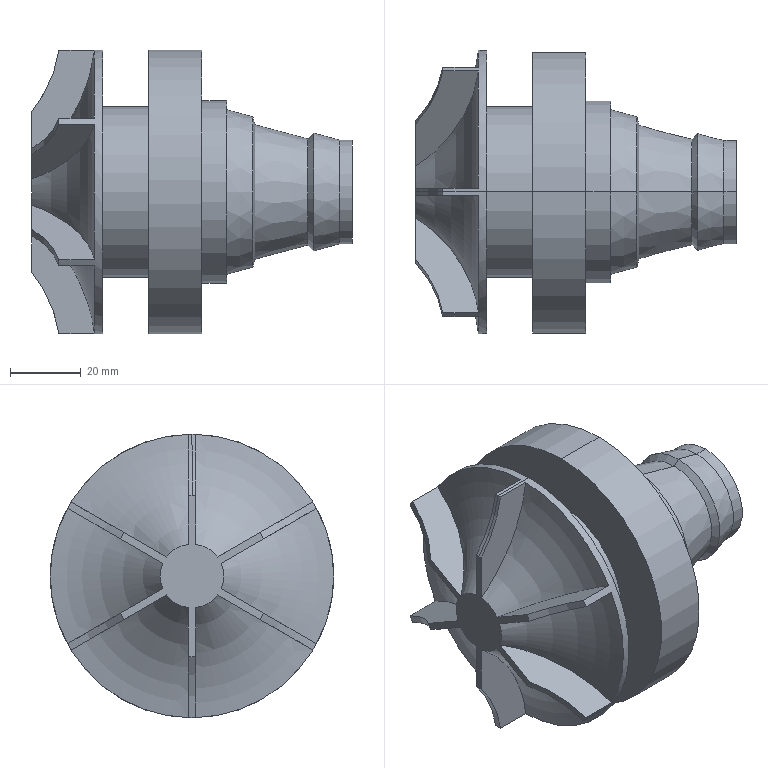Part | SolidWorks | features ICE 2, HoleWzd 1, RevCut 1, Revolution 1 | 1 solid | 62 faces | box 90.5 x 80 x 80 mm | volume 181768 mm3 | plane 22 | cylinder 15 | torus 13 | cone 12 | commonest cylinder face diameters 80 x5 10.5 x2 18 x2 29.3 x2 48 x2 51.5 x2